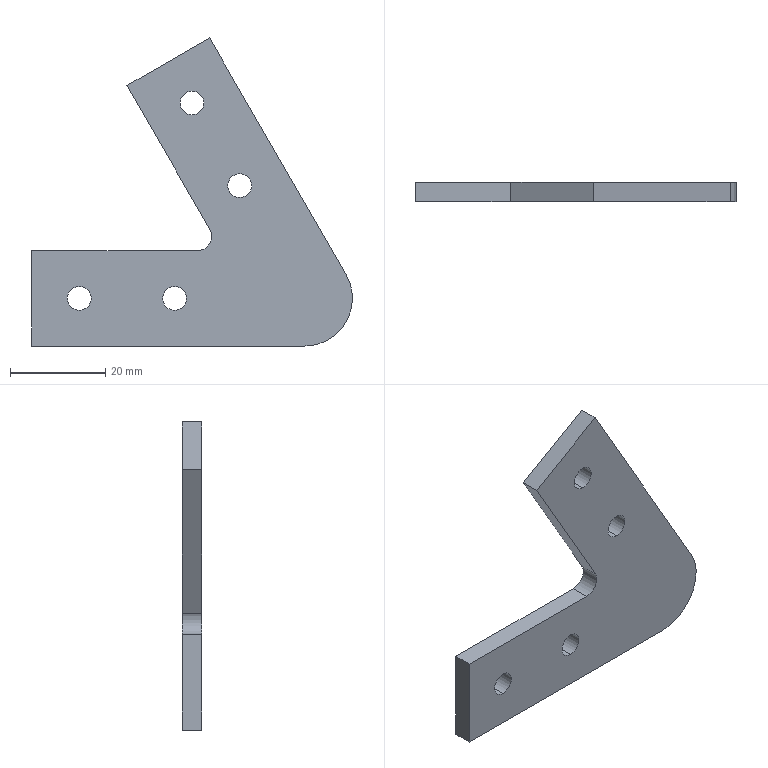Part | STEP file | 60-degree side frame | 1 solid | 18 faces | box 67.321 x 4 x 64.641 mm | volume 8608 mm3 | cylinder 10 | plane 8 | commonest cylinder face diameters 5 x8 6 x1 20 x1